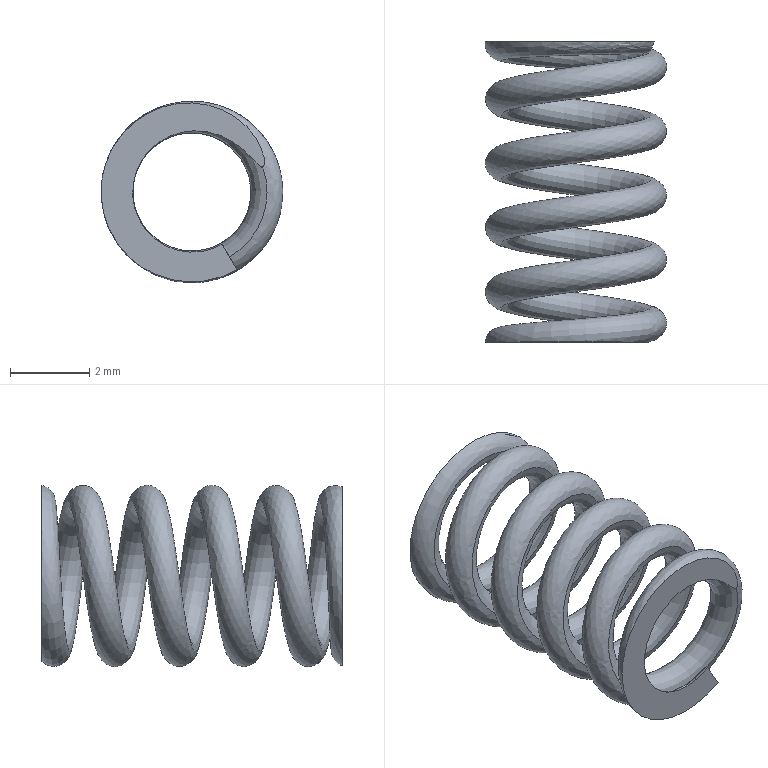Part | SolidWorks | features BaseBody 1 | 1 solid | 6 faces | volume 30.226 mm3 | plane 4 | spline 2